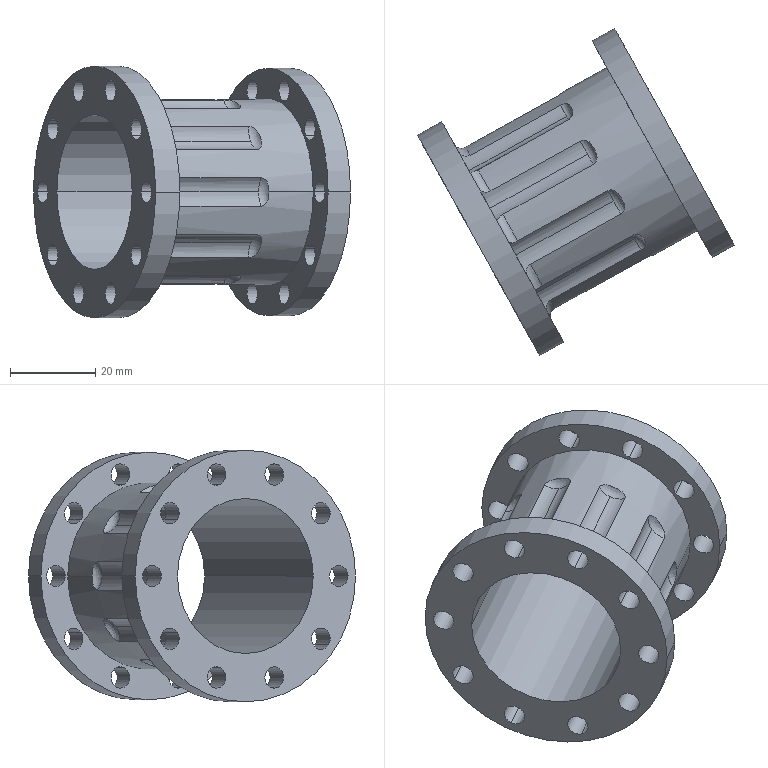Part | STEP file | Completa.sldasm-Part-29_Valor predeterminado | 1 solid | 92 faces | box 74.277 x 76.616 x 59 mm | volume 34566 mm3 | cylinder 68 | torus 20 | plane 4 | commonest cylinder face diameters 5 x40 9.5 x20 36.376 x2 43.646 x2 58 x2 59 x2